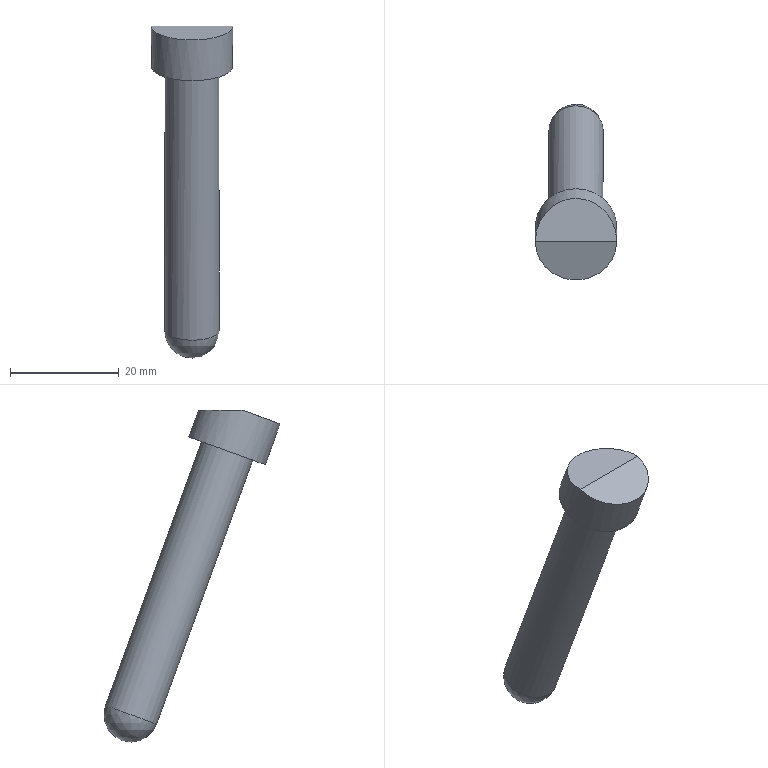Part | STEP file | lll_id286_x_t | 1 solid | 6 faces | box 15 x 32.483 x 61.146 mm | volume 5638 mm3 | plane 3 | cylinder 2 | sphere 1 | commonest cylinder face diameters 10 x1 15 x1
STEP:
#1=CARTESIAN_POINT('',(7.5,111.066,30.));
#2=VERTEX_POINT('',#1);
#3=CARTESIAN_POINT('',(-7.5,111.066,30.));
#4=VERTEX_POINT('',#3);
#5=CARTESIAN_POINT('',(0.,111.066,30.));
#6=DIRECTION('',(0.,0.342,-0.9397));
#7=DIRECTION('',(0.,-0.9397,-0.342));
#8=AXIS2_PLACEMENT_3D('',#5,#6,#7);
#9=CIRCLE('',#8,7.5);
#10=EDGE_CURVE('',#2,#4,#9,.T.);
#11=ORIENTED_EDGE('',*,*,#10,.F.);
#12=CARTESIAN_POINT('',(0.,111.066,30.));
#13=DIRECTION('',(-1.,0.,0.));
#14=VECTOR('',#13,1.);
#15=LINE('',#12,#14);
#16=EDGE_CURVE('',#2,#4,#15,.T.);
#17=ORIENTED_EDGE('',*,*,#16,.T.);
#18=EDGE_LOOP('',(#11,#17));
#19=FACE_OUTER_BOUND('',#18,.T.);
#20=CARTESIAN_POINT('',(0.,111.066,30.));
#21=DIRECTION('',(0.,-0.342,0.9397));
#22=DIRECTION('',(0.,0.9397,0.342));
#23=AXIS2_PLACEMENT_3D('',#20,#21,#22);
#24=PLANE('',#23);
#25=ADVANCED_FACE('',(#19),#24,.T.);
#26=CARTESIAN_POINT('',(0.,120.85,25.048));
#27=VERTEX_POINT('',#26);
#28=CARTESIAN_POINT('',(0.,113.802,22.482));
#29=DIRECTION('',(0.,-0.342,0.9397));
#30=DIRECTION('',(0.,0.9397,0.342));
#31=AXIS2_PLACEMENT_3D('',#28,#29,#30);
#32=CIRCLE('',#31,7.5);
#33=EDGE_CURVE('',#27,#27,#32,.T.);
#34=ORIENTED_EDGE('',*,*,#33,.T.);
#35=EDGE_LOOP('',(#34));
#36=FACE_BOUND('',#35,.T.);
#37=ORIENTED_EDGE('',*,*,#10,.T.);
#38=CARTESIAN_POINT('',(0.,111.066,30.));
#39=DIRECTION('',(0.,0.,-1.));
#40=DIRECTION('',(0.,-1.,0.));
#41=AXIS2_PLACEMENT_3D('',#38,#39,#40);
#42=ELLIPSE('',#41,7.981,7.5);
#43=EDGE_CURVE('',#4,#2,#42,.T.);
#44=ORIENTED_EDGE('',*,*,#43,.T.);
#45=EDGE_LOOP('',(#37,#44));
#46=FACE_BOUND('',#45,.T.);
#47=CARTESIAN_POINT('',(0.,113.802,22.482));
#48=DIRECTION('',(0.,-0.342,0.9397));
#49=DIRECTION('',(0.,0.9397,0.342));
#50=AXIS2_PLACEMENT_3D('',#47,#48,#49);
#51=CYLINDRICAL_SURFACE('',#50,7.5);
#52=ADVANCED_FACE('',(#36,#46),#51,.T.);
#53=CARTESIAN_POINT('',(0.,136.2,-24.436));
#54=VERTEX_POINT('',#53);
#55=CARTESIAN_POINT('',(0.,131.502,-26.146));
#56=DIRECTION('',(0.,-0.342,0.9397));
#57=DIRECTION('',(0.,0.9397,0.342));
#58=AXIS2_PLACEMENT_3D('',#55,#56,#57);
#59=CIRCLE('',#58,5.);
#60=EDGE_CURVE('',#54,#54,#59,.T.);
#61=ORIENTED_EDGE('',*,*,#60,.T.);
#62=EDGE_LOOP('',(#61));
#63=FACE_BOUND('',#62,.T.);
#64=CARTESIAN_POINT('',(0.,109.104,20.772));
#65=VERTEX_POINT('',#64);
#66=CARTESIAN_POINT('',(0.,113.802,22.482));
#67=DIRECTION('',(0.,-0.342,0.9397));
#68=DIRECTION('',(0.,-0.9397,-0.342));
#69=AXIS2_PLACEMENT_3D('',#66,#67,#68);
#70=CIRCLE('',#69,5.);
#71=EDGE_CURVE('',#65,#65,#70,.T.);
#72=ORIENTED_EDGE('',*,*,#71,.F.);
#73=EDGE_LOOP('',(#72));
#74=FACE_BOUND('',#73,.T.);
#75=CARTESIAN_POINT('',(0.,138.,-44.));
#76=DIRECTION('',(0.,-0.342,0.9397));
#77=DIRECTION('',(-1.,0.,0.));
#78=AXIS2_PLACEMENT_3D('',#75,#76,#77);
#79=CYLINDRICAL_SURFACE('',#78,5.);
#80=ADVANCED_FACE('',(#63,#74),#79,.T.);
#81=ORIENTED_EDGE('',*,*,#71,.T.);
#82=EDGE_LOOP('',(#81));
#83=FACE_BOUND('',#82,.T.);
#84=ORIENTED_EDGE('',*,*,#33,.F.);
#85=EDGE_LOOP('',(#84));
#86=FACE_BOUND('',#85,.T.);
#87=CARTESIAN_POINT('',(0.,113.802,22.482));
#88=DIRECTION('',(0.,0.342,-0.9397));
#89=DIRECTION('',(0.,-0.9397,-0.342));
#90=AXIS2_PLACEMENT_3D('',#87,#88,#89);
#91=PLANE('',#90);
#92=ADVANCED_FACE('',(#83,#86),#91,.T.);
#93=ORIENTED_EDGE('',*,*,#16,.F.);
#94=ORIENTED_EDGE('',*,*,#43,.F.);
#95=EDGE_LOOP('',(#93,#94));
#96=FACE_OUTER_BOUND('',#95,.T.);
#97=CARTESIAN_POINT('',(0.,115.5,30.));
#98=DIRECTION('',(0.,0.,1.));
#99=DIRECTION('',(-1.,0.,0.));
#100=AXIS2_PLACEMENT_3D('',#97,#98,#99);
#101=PLANE('',#100);
#102=ADVANCED_FACE('',(#96),#101,.T.);
#103=ORIENTED_EDGE('',*,*,#60,.F.);
#104=EDGE_LOOP('',(#103));
#105=FACE_OUTER_BOUND('',#104,.T.);
#106=CARTESIAN_POINT('',(0.,131.502,-26.146));
#107=DIRECTION('',(0.,0.,1.));
#108=DIRECTION('',(-1.,0.,0.));
#109=AXIS2_PLACEMENT_3D('',#106,#107,#108);
#110=SPHERICAL_SURFACE('',#109,5.);
#111=ADVANCED_FACE('',(#105),#110,.T.);
#112=CLOSED_SHELL('',(#25,#52,#80,#92,#102,#111));
#113=MANIFOLD_SOLID_BREP('',#112);
#114=(LENGTH_UNIT()NAMED_UNIT(*)SI_UNIT(.MILLI.,.METRE.));
#115=UNCERTAINTY_MEASURE_WITH_UNIT(LENGTH_MEASURE(0.00002),#114,'','');
#116=(NAMED_UNIT(*)PLANE_ANGLE_UNIT()SI_UNIT($,.RADIAN.));
#117=PLANE_ANGLE_MEASURE_WITH_UNIT(PLANE_ANGLE_MEASURE(0.01745),#116);
#118=DIMENSIONAL_EXPONENTS(0.,0.,0.,0.,0.,0.,0.);
#119=(CONVERSION_BASED_UNIT('DEGREE',#117)NAMED_UNIT(#118)PLANE_ANGLE_UNIT());
#120=(NAMED_UNIT(*)SI_UNIT($,.STERADIAN.)SOLID_ANGLE_UNIT());
#121=(GEOMETRIC_REPRESENTATION_CONTEXT(3)GLOBAL_UNCERTAINTY_ASSIGNED_CONTEXT((#115))GLOBAL_UNIT_ASSIGNED_CONTEXT((#114,#119,#120))REPRESENTATION_CONTEXT('',''));
#122=ADVANCED_BREP_SHAPE_REPRESENTATION('',(#113),#121);